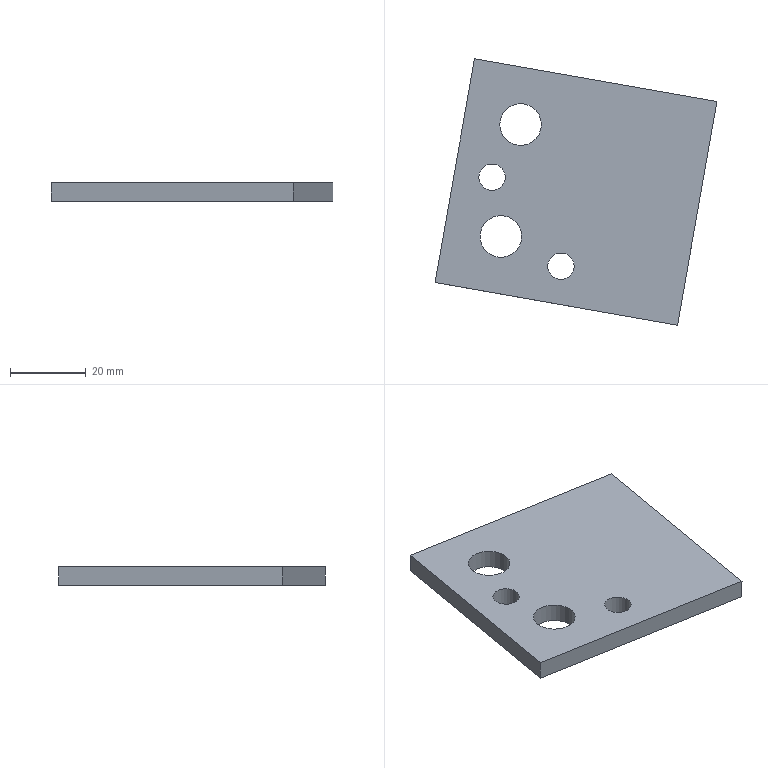Part | NX | features solid 2 | 1 solid | 10 faces | box 74.431 x 70.376 x 5 mm | volume 18165 mm3 | plane 6 | cylinder 4 | commonest cylinder face diameters 7 x2 11 x2
STEP:
#1=CARTESIAN_POINT('',(407.426,134.834,68.192));
#2=VERTEX_POINT('',#1);
#3=CARTESIAN_POINT('',(471.438,123.547,68.192));
#4=VERTEX_POINT('',#3);
#5=CARTESIAN_POINT('',(405.456,135.181,68.192));
#6=DIRECTION('',(-0.9848,0.1736,0.000000468));
#7=VECTOR('',#6,1000.);
#8=LINE('',#5,#7);
#9=EDGE_CURVE('',#2,#4,#8,.F.);
#10=ORIENTED_EDGE('',*,*,#9,.F.);
#11=CARTESIAN_POINT('',(407.426,134.834,63.192));
#12=VERTEX_POINT('',#11);
#13=CARTESIAN_POINT('',(407.426,134.834,63.192));
#14=DIRECTION('',(0.000000502,0.000000149,1.));
#15=VECTOR('',#14,1000.);
#16=LINE('',#13,#15);
#17=EDGE_CURVE('',#12,#2,#16,.T.);
#18=ORIENTED_EDGE('',*,*,#17,.F.);
#19=CARTESIAN_POINT('',(471.438,123.547,63.192));
#20=VERTEX_POINT('',#19);
#21=CARTESIAN_POINT('',(405.456,135.181,63.192));
#22=DIRECTION('',(-0.9848,0.1736,0.000000468));
#23=VECTOR('',#22,1000.);
#24=LINE('',#21,#23);
#25=EDGE_CURVE('',#12,#20,#24,.F.);
#26=ORIENTED_EDGE('',*,*,#25,.T.);
#27=CARTESIAN_POINT('',(471.438,123.547,63.192));
#28=DIRECTION('',(0.000000502,0.000000149,1.));
#29=VECTOR('',#28,1000.);
#30=LINE('',#27,#29);
#31=EDGE_CURVE('',#20,#4,#30,.T.);
#32=ORIENTED_EDGE('',*,*,#31,.T.);
#33=EDGE_LOOP('',(#10,#18,#26,#32));
#34=FACE_BOUND('',#33,.T.);
#35=CARTESIAN_POINT('',(405.456,135.181,63.192));
#36=DIRECTION('',(0.1736,0.9848,-0.000000234));
#37=DIRECTION('',(0.9848,-0.1736,-0.000000468));
#38=AXIS2_PLACEMENT_3D('',#35,#36,#37);
#39=PLANE('',#38);
#40=ADVANCED_FACE('',(#34),#39,.F.);
#41=CARTESIAN_POINT('',(417.845,193.923,68.192));
#42=VERTEX_POINT('',#41);
#43=CARTESIAN_POINT('',(418.713,198.847,68.192));
#44=DIRECTION('',(0.1736,0.9848,-0.000000234));
#45=VECTOR('',#44,1000.);
#46=LINE('',#43,#45);
#47=EDGE_CURVE('',#42,#2,#46,.F.);
#48=ORIENTED_EDGE('',*,*,#47,.F.);
#49=CARTESIAN_POINT('',(417.845,193.923,63.192));
#50=VERTEX_POINT('',#49);
#51=CARTESIAN_POINT('',(417.845,193.923,63.192));
#52=DIRECTION('',(0.000000502,0.000000149,1.));
#53=VECTOR('',#52,1000.);
#54=LINE('',#51,#53);
#55=EDGE_CURVE('',#50,#42,#54,.T.);
#56=ORIENTED_EDGE('',*,*,#55,.F.);
#57=CARTESIAN_POINT('',(418.713,198.847,63.192));
#58=DIRECTION('',(0.1736,0.9848,-0.000000234));
#59=VECTOR('',#58,1000.);
#60=LINE('',#57,#59);
#61=EDGE_CURVE('',#50,#12,#60,.F.);
#62=ORIENTED_EDGE('',*,*,#61,.T.);
#63=ORIENTED_EDGE('',*,*,#17,.T.);
#64=EDGE_LOOP('',(#48,#56,#62,#63));
#65=FACE_BOUND('',#64,.T.);
#66=CARTESIAN_POINT('',(418.713,198.847,63.192));
#67=DIRECTION('',(0.9848,-0.1736,-0.000000468));
#68=DIRECTION('',(-0.1736,-0.9848,0.000000234));
#69=AXIS2_PLACEMENT_3D('',#66,#67,#68);
#70=PLANE('',#69);
#71=ADVANCED_FACE('',(#65),#70,.F.);
#72=CARTESIAN_POINT('',(481.857,182.635,68.192));
#73=VERTEX_POINT('',#72);
#74=CARTESIAN_POINT('',(415.875,194.27,68.192));
#75=DIRECTION('',(0.9848,-0.1736,-0.000000468));
#76=VECTOR('',#75,1000.);
#77=LINE('',#74,#76);
#78=EDGE_CURVE('',#73,#42,#77,.F.);
#79=ORIENTED_EDGE('',*,*,#78,.F.);
#80=CARTESIAN_POINT('',(481.857,182.635,63.192));
#81=VERTEX_POINT('',#80);
#82=CARTESIAN_POINT('',(481.857,182.635,63.192));
#83=DIRECTION('',(0.000000502,0.000000149,1.));
#84=VECTOR('',#83,1000.);
#85=LINE('',#82,#84);
#86=EDGE_CURVE('',#81,#73,#85,.T.);
#87=ORIENTED_EDGE('',*,*,#86,.F.);
#88=CARTESIAN_POINT('',(415.875,194.27,63.192));
#89=DIRECTION('',(0.9848,-0.1736,-0.000000468));
#90=VECTOR('',#89,1000.);
#91=LINE('',#88,#90);
#92=EDGE_CURVE('',#81,#50,#91,.F.);
#93=ORIENTED_EDGE('',*,*,#92,.T.);
#94=ORIENTED_EDGE('',*,*,#55,.T.);
#95=EDGE_LOOP('',(#79,#87,#93,#94));
#96=FACE_BOUND('',#95,.T.);
#97=CARTESIAN_POINT('',(415.875,194.27,63.192));
#98=DIRECTION('',(-0.1736,-0.9848,0.000000234));
#99=DIRECTION('',(-0.9848,0.1736,0.000000468));
#100=AXIS2_PLACEMENT_3D('',#97,#98,#99);
#101=PLANE('',#100);
#102=ADVANCED_FACE('',(#96),#101,.F.);
#103=CARTESIAN_POINT('',(482.726,187.559,68.192));
#104=DIRECTION('',(-0.1736,-0.9848,0.000000234));
#105=VECTOR('',#104,1000.);
#106=LINE('',#103,#105);
#107=EDGE_CURVE('',#4,#73,#106,.F.);
#108=ORIENTED_EDGE('',*,*,#107,.F.);
#109=ORIENTED_EDGE('',*,*,#31,.F.);
#110=CARTESIAN_POINT('',(482.726,187.559,63.192));
#111=DIRECTION('',(-0.1736,-0.9848,0.000000234));
#112=VECTOR('',#111,1000.);
#113=LINE('',#110,#112);
#114=EDGE_CURVE('',#20,#81,#113,.F.);
#115=ORIENTED_EDGE('',*,*,#114,.T.);
#116=ORIENTED_EDGE('',*,*,#86,.T.);
#117=EDGE_LOOP('',(#108,#109,#115,#116));
#118=FACE_BOUND('',#117,.T.);
#119=CARTESIAN_POINT('',(482.726,187.559,63.192));
#120=DIRECTION('',(-0.9848,0.1736,0.000000468));
#121=DIRECTION('',(0.1736,0.9848,-0.000000234));
#122=AXIS2_PLACEMENT_3D('',#119,#120,#121);
#123=PLANE('',#122);
#124=ADVANCED_FACE('',(#118),#123,.F.);
#125=CARTESIAN_POINT('',(435.512,176.546,63.192));
#126=VERTEX_POINT('',#125);
#127=CARTESIAN_POINT('',(430.012,176.546,63.192));
#128=DIRECTION('',(0.000000502,0.000000149,1.));
#129=DIRECTION('',(1.,-0.000001668,-0.000000502));
#130=AXIS2_PLACEMENT_3D('',#127,#128,#129);
#131=CIRCLE('',#130,5.5);
#132=EDGE_CURVE('',#126,#126,#131,.F.);
#133=ORIENTED_EDGE('',*,*,#132,.T.);
#134=EDGE_LOOP('',(#133));
#135=FACE_BOUND('',#134,.T.);
#136=CARTESIAN_POINT('',(435.512,176.546,68.192));
#137=VERTEX_POINT('',#136);
#138=CARTESIAN_POINT('',(430.012,176.546,68.192));
#139=DIRECTION('',(0.000000502,0.000000149,1.));
#140=DIRECTION('',(1.,-0.000001668,-0.000000502));
#141=AXIS2_PLACEMENT_3D('',#138,#139,#140);
#142=CIRCLE('',#141,5.5);
#143=EDGE_CURVE('',#137,#137,#142,.F.);
#144=ORIENTED_EDGE('',*,*,#143,.F.);
#145=EDGE_LOOP('',(#144));
#146=FACE_BOUND('',#145,.T.);
#147=CARTESIAN_POINT('',(430.012,176.546,63.192));
#148=DIRECTION('',(0.000000502,0.000000149,1.));
#149=DIRECTION('',(-1.,0.000001668,0.000000502));
#150=AXIS2_PLACEMENT_3D('',#147,#148,#149);
#151=CYLINDRICAL_SURFACE('',#150,5.5);
#152=ADVANCED_FACE('',(#135,#146),#151,.F.);
#153=CARTESIAN_POINT('',(430.303,147.002,63.192));
#154=VERTEX_POINT('',#153);
#155=CARTESIAN_POINT('',(424.803,147.002,63.192));
#156=DIRECTION('',(0.000000502,0.000000149,1.));
#157=DIRECTION('',(1.,-0.000001668,-0.000000502));
#158=AXIS2_PLACEMENT_3D('',#155,#156,#157);
#159=CIRCLE('',#158,5.5);
#160=EDGE_CURVE('',#154,#154,#159,.F.);
#161=ORIENTED_EDGE('',*,*,#160,.T.);
#162=EDGE_LOOP('',(#161));
#163=FACE_BOUND('',#162,.T.);
#164=CARTESIAN_POINT('',(430.303,147.002,68.192));
#165=VERTEX_POINT('',#164);
#166=CARTESIAN_POINT('',(424.803,147.002,68.192));
#167=DIRECTION('',(0.000000502,0.000000149,1.));
#168=DIRECTION('',(1.,-0.000001668,-0.000000502));
#169=AXIS2_PLACEMENT_3D('',#166,#167,#168);
#170=CIRCLE('',#169,5.5);
#171=EDGE_CURVE('',#165,#165,#170,.F.);
#172=ORIENTED_EDGE('',*,*,#171,.F.);
#173=EDGE_LOOP('',(#172));
#174=FACE_BOUND('',#173,.T.);
#175=CARTESIAN_POINT('',(424.803,147.002,63.192));
#176=DIRECTION('',(0.000000502,0.000000149,1.));
#177=DIRECTION('',(-1.,0.000001668,0.000000502));
#178=AXIS2_PLACEMENT_3D('',#175,#176,#177);
#179=CYLINDRICAL_SURFACE('',#178,5.5);
#180=ADVANCED_FACE('',(#163,#174),#179,.F.);
#181=CARTESIAN_POINT('',(425.984,162.642,63.192));
#182=VERTEX_POINT('',#181);
#183=CARTESIAN_POINT('',(422.484,162.642,63.192));
#184=DIRECTION('',(0.000000502,0.000000149,1.));
#185=DIRECTION('',(1.,0.,-0.000000502));
#186=AXIS2_PLACEMENT_3D('',#183,#184,#185);
#187=CIRCLE('',#186,3.5);
#188=EDGE_CURVE('',#182,#182,#187,.F.);
#189=ORIENTED_EDGE('',*,*,#188,.T.);
#190=EDGE_LOOP('',(#189));
#191=FACE_BOUND('',#190,.T.);
#192=CARTESIAN_POINT('',(425.984,162.642,68.192));
#193=VERTEX_POINT('',#192);
#194=CARTESIAN_POINT('',(422.484,162.642,68.192));
#195=DIRECTION('',(0.000000502,0.000000149,1.));
#196=DIRECTION('',(1.,0.,-0.000000502));
#197=AXIS2_PLACEMENT_3D('',#194,#195,#196);
#198=CIRCLE('',#197,3.5);
#199=EDGE_CURVE('',#193,#193,#198,.F.);
#200=ORIENTED_EDGE('',*,*,#199,.F.);
#201=EDGE_LOOP('',(#200));
#202=FACE_BOUND('',#201,.T.);
#203=CARTESIAN_POINT('',(422.484,162.642,63.192));
#204=DIRECTION('',(0.000000502,0.000000149,1.));
#205=DIRECTION('',(-1.,0.000001668,0.000000502));
#206=AXIS2_PLACEMENT_3D('',#203,#204,#205);
#207=CYLINDRICAL_SURFACE('',#206,3.5);
#208=ADVANCED_FACE('',(#191,#202),#207,.F.);
#209=CARTESIAN_POINT('',(444.176,139.125,63.192));
#210=VERTEX_POINT('',#209);
#211=CARTESIAN_POINT('',(440.676,139.125,63.192));
#212=DIRECTION('',(0.000000502,0.000000149,1.));
#213=DIRECTION('',(1.,0.,-0.000000502));
#214=AXIS2_PLACEMENT_3D('',#211,#212,#213);
#215=CIRCLE('',#214,3.5);
#216=EDGE_CURVE('',#210,#210,#215,.F.);
#217=ORIENTED_EDGE('',*,*,#216,.T.);
#218=EDGE_LOOP('',(#217));
#219=FACE_BOUND('',#218,.T.);
#220=CARTESIAN_POINT('',(444.176,139.125,68.192));
#221=VERTEX_POINT('',#220);
#222=CARTESIAN_POINT('',(440.676,139.125,68.192));
#223=DIRECTION('',(0.000000502,0.000000149,1.));
#224=DIRECTION('',(1.,0.,-0.000000502));
#225=AXIS2_PLACEMENT_3D('',#222,#223,#224);
#226=CIRCLE('',#225,3.5);
#227=EDGE_CURVE('',#221,#221,#226,.F.);
#228=ORIENTED_EDGE('',*,*,#227,.F.);
#229=EDGE_LOOP('',(#228));
#230=FACE_BOUND('',#229,.T.);
#231=CARTESIAN_POINT('',(440.676,139.125,63.192));
#232=DIRECTION('',(0.000000502,0.000000149,1.));
#233=DIRECTION('',(-1.,0.000001668,0.000000502));
#234=AXIS2_PLACEMENT_3D('',#231,#232,#233);
#235=CYLINDRICAL_SURFACE('',#234,3.5);
#236=ADVANCED_FACE('',(#219,#230),#235,.F.);
#237=ORIENTED_EDGE('',*,*,#216,.F.);
#238=EDGE_LOOP('',(#237));
#239=FACE_BOUND('',#238,.T.);
#240=ORIENTED_EDGE('',*,*,#188,.F.);
#241=EDGE_LOOP('',(#240));
#242=FACE_BOUND('',#241,.T.);
#243=ORIENTED_EDGE('',*,*,#160,.F.);
#244=EDGE_LOOP('',(#243));
#245=FACE_BOUND('',#244,.T.);
#246=ORIENTED_EDGE('',*,*,#132,.F.);
#247=EDGE_LOOP('',(#246));
#248=FACE_BOUND('',#247,.T.);
#249=ORIENTED_EDGE('',*,*,#25,.F.);
#250=ORIENTED_EDGE('',*,*,#61,.F.);
#251=ORIENTED_EDGE('',*,*,#92,.F.);
#252=ORIENTED_EDGE('',*,*,#114,.F.);
#253=EDGE_LOOP('',(#249,#250,#251,#252));
#254=FACE_BOUND('',#253,.T.);
#255=CARTESIAN_POINT('',(486.873,147.734,63.192));
#256=DIRECTION('',(-0.000000502,-0.000000149,-1.));
#257=DIRECTION('',(0.9848,-0.1736,-0.000000468));
#258=AXIS2_PLACEMENT_3D('',#255,#256,#257);
#259=PLANE('',#258);
#260=ADVANCED_FACE('',(#239,#242,#245,#248,#254),#259,.T.);
#261=ORIENTED_EDGE('',*,*,#227,.T.);
#262=EDGE_LOOP('',(#261));
#263=FACE_BOUND('',#262,.T.);
#264=ORIENTED_EDGE('',*,*,#199,.T.);
#265=EDGE_LOOP('',(#264));
#266=FACE_BOUND('',#265,.T.);
#267=ORIENTED_EDGE('',*,*,#171,.T.);
#268=EDGE_LOOP('',(#267));
#269=FACE_BOUND('',#268,.T.);
#270=ORIENTED_EDGE('',*,*,#143,.T.);
#271=EDGE_LOOP('',(#270));
#272=FACE_BOUND('',#271,.T.);
#273=ORIENTED_EDGE('',*,*,#9,.T.);
#274=ORIENTED_EDGE('',*,*,#107,.T.);
#275=ORIENTED_EDGE('',*,*,#78,.T.);
#276=ORIENTED_EDGE('',*,*,#47,.T.);
#277=EDGE_LOOP('',(#273,#274,#275,#276));
#278=FACE_BOUND('',#277,.T.);
#279=CARTESIAN_POINT('',(486.873,147.734,68.192));
#280=DIRECTION('',(-0.000000502,-0.000000149,-1.));
#281=DIRECTION('',(0.9848,-0.1736,-0.000000468));
#282=AXIS2_PLACEMENT_3D('',#279,#280,#281);
#283=PLANE('',#282);
#284=ADVANCED_FACE('',(#263,#266,#269,#272,#278),#283,.F.);
#285=CLOSED_SHELL('',(#40,#71,#102,#124,#152,#180,#208,#236,#260,#284));
#286=MANIFOLD_SOLID_BREP('',#285);
#287=(LENGTH_UNIT()NAMED_UNIT(*)SI_UNIT(.MILLI.,.METRE.));
#288=UNCERTAINTY_MEASURE_WITH_UNIT(LENGTH_MEASURE(0.00001),#287,'','');
#289=(NAMED_UNIT(*)PLANE_ANGLE_UNIT()SI_UNIT($,.RADIAN.));
#290=(NAMED_UNIT(*)SI_UNIT($,.STERADIAN.)SOLID_ANGLE_UNIT());
#291=(GEOMETRIC_REPRESENTATION_CONTEXT(3)GLOBAL_UNCERTAINTY_ASSIGNED_CONTEXT((#288))GLOBAL_UNIT_ASSIGNED_CONTEXT((#287,#289,#290))REPRESENTATION_CONTEXT('',''));
#292=ADVANCED_BREP_SHAPE_REPRESENTATION('',(#286),#291);